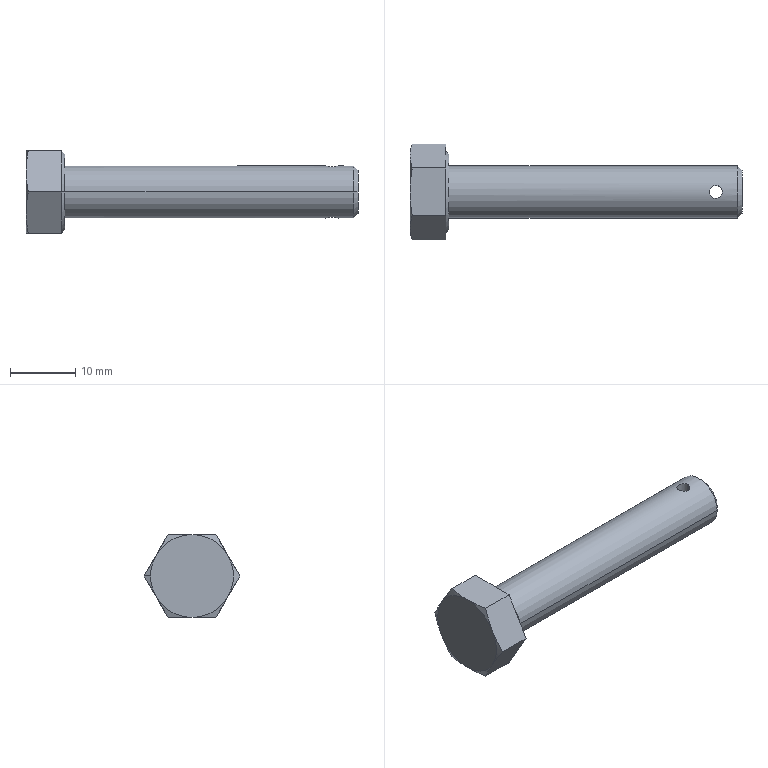Part | SolidWorks | features BaseBody 1 | 1 solid | 30 faces | box 50.95 x 14.699 x 12.73 mm | volume 3053 mm3 | plane 15 | cone 11 | cylinder 4 | commonest cylinder face diameters 2 x2 8 x2
STEP:
#1=CARTESIAN_POINT('',(45.95,0.,-4.));
#2=VERTEX_POINT('',#1);
#3=CARTESIAN_POINT('',(47.95,0.,-4.));
#4=VERTEX_POINT('',#3);
#5=CARTESIAN_POINT('',(45.95,0.,-4.));
#6=CARTESIAN_POINT('',(45.95,-0.1327,-4.));
#7=CARTESIAN_POINT('',(45.976,-0.2612,-3.993));
#8=CARTESIAN_POINT('',(46.077,-0.5055,-3.97));
#9=CARTESIAN_POINT('',(46.149,-0.6129,-3.954));
#10=CARTESIAN_POINT('',(46.336,-0.8007,-3.92));
#11=CARTESIAN_POINT('',(46.443,-0.8722,-3.904));
#12=CARTESIAN_POINT('',(46.689,-0.9745,-3.88));
#13=CARTESIAN_POINT('',(46.817,-0.9999,-3.873));
#14=CARTESIAN_POINT('',(47.082,-1.,-3.873));
#15=CARTESIAN_POINT('',(47.212,-0.9741,-3.88));
#16=CARTESIAN_POINT('',(47.455,-0.8731,-3.904));
#17=CARTESIAN_POINT('',(47.563,-0.8008,-3.92));
#18=CARTESIAN_POINT('',(47.75,-0.6142,-3.954));
#19=CARTESIAN_POINT('',(47.822,-0.5075,-3.97));
#20=CARTESIAN_POINT('',(47.924,-0.2615,-3.993));
#21=CARTESIAN_POINT('',(47.95,-0.1331,-4.));
#22=CARTESIAN_POINT('',(47.95,0.,-4.));
#23=B_SPLINE_CURVE_WITH_KNOTS('',3,(#5,#6,#7,#8,#9,#10,#11,#12,#13,#14,#15,#16,#17,#18,#19,#20,#21,#22),.UNSPECIFIED.,.F.,.F.,(4,2,2,2,2,2,2,2,4),(0.,0.125,0.25,0.375,0.5,0.625,0.75,0.875,1.),.UNSPECIFIED.);
#24=EDGE_CURVE('',#2,#4,#23,.T.);
#25=ORIENTED_EDGE('',*,*,#24,.F.);
#26=CARTESIAN_POINT('',(45.95,0.,4.));
#27=VERTEX_POINT('',#26);
#28=CARTESIAN_POINT('',(45.95,0.,-6.365));
#29=DIRECTION('',(0.,0.,1.));
#30=VECTOR('',#29,1000.);
#31=LINE('',#28,#30);
#32=EDGE_CURVE('',#2,#27,#31,.T.);
#33=ORIENTED_EDGE('',*,*,#32,.T.);
#34=CARTESIAN_POINT('',(47.95,0.,4.));
#35=VERTEX_POINT('',#34);
#36=CARTESIAN_POINT('',(47.95,0.,4.));
#37=CARTESIAN_POINT('',(47.95,-0.1329,4.));
#38=CARTESIAN_POINT('',(47.924,-0.2617,3.993));
#39=CARTESIAN_POINT('',(47.823,-0.5061,3.97));
#40=CARTESIAN_POINT('',(47.751,-0.6136,3.954));
#41=CARTESIAN_POINT('',(47.563,-0.8011,3.92));
#42=CARTESIAN_POINT('',(47.456,-0.8725,3.904));
#43=CARTESIAN_POINT('',(47.211,-0.9745,3.88));
#44=CARTESIAN_POINT('',(47.083,-0.9999,3.873));
#45=CARTESIAN_POINT('',(46.818,-1.,3.873));
#46=CARTESIAN_POINT('',(46.689,-0.9742,3.88));
#47=CARTESIAN_POINT('',(46.445,-0.873,3.904));
#48=CARTESIAN_POINT('',(46.336,-0.8005,3.92));
#49=CARTESIAN_POINT('',(46.149,-0.6134,3.954));
#50=CARTESIAN_POINT('',(46.077,-0.506,3.97));
#51=CARTESIAN_POINT('',(45.975,-0.2607,3.993));
#52=CARTESIAN_POINT('',(45.95,-0.1327,4.));
#53=CARTESIAN_POINT('',(45.95,0.,4.));
#54=B_SPLINE_CURVE_WITH_KNOTS('',3,(#36,#37,#38,#39,#40,#41,#42,#43,#44,#45,#46,#47,#48,#49,#50,#51,#52,#53),.UNSPECIFIED.,.F.,.F.,(4,2,2,2,2,2,2,2,4),(0.,0.125,0.25,0.375,0.5,0.625,0.75,0.875,1.),.UNSPECIFIED.);
#55=EDGE_CURVE('',#35,#27,#54,.T.);
#56=ORIENTED_EDGE('',*,*,#55,.F.);
#57=CARTESIAN_POINT('',(47.95,0.,-6.365));
#58=DIRECTION('',(0.,0.,1.));
#59=VECTOR('',#58,1000.);
#60=LINE('',#57,#59);
#61=EDGE_CURVE('',#4,#35,#60,.T.);
#62=ORIENTED_EDGE('',*,*,#61,.F.);
#63=EDGE_LOOP('',(#25,#33,#56,#62));
#64=FACE_OUTER_BOUND('',#63,.T.);
#65=CARTESIAN_POINT('',(46.95,0.,-6.365));
#66=DIRECTION('',(0.,0.,1.));
#67=DIRECTION('',(1.,0.,0.));
#68=AXIS2_PLACEMENT_3D('',#65,#66,#67);
#69=CYLINDRICAL_SURFACE('',#68,1.);
#70=ADVANCED_FACE('',(#64),#69,.F.);
#71=CARTESIAN_POINT('',(50.95,3.324,0.));
#72=VERTEX_POINT('',#71);
#73=CARTESIAN_POINT('',(50.95,-3.324,0.));
#74=VERTEX_POINT('',#73);
#75=CARTESIAN_POINT('',(50.95,0.,0.));
#76=DIRECTION('',(1.,0.,0.));
#77=DIRECTION('',(0.,1.,0.));
#78=AXIS2_PLACEMENT_3D('',#75,#76,#77);
#79=CIRCLE('',#78,3.324);
#80=EDGE_CURVE('',#72,#74,#79,.T.);
#81=ORIENTED_EDGE('',*,*,#80,.F.);
#82=CARTESIAN_POINT('',(50.273,4.,0.));
#83=VERTEX_POINT('',#82);
#84=CARTESIAN_POINT('',(50.95,3.324,0.));
#85=DIRECTION('',(-0.7071,0.7071,0.));
#86=VECTOR('',#85,1000.);
#87=LINE('',#84,#86);
#88=EDGE_CURVE('',#72,#83,#87,.T.);
#89=ORIENTED_EDGE('',*,*,#88,.T.);
#90=CARTESIAN_POINT('',(50.273,-4.,0.));
#91=VERTEX_POINT('',#90);
#92=CARTESIAN_POINT('',(50.273,0.,0.));
#93=DIRECTION('',(-1.,0.,0.));
#94=DIRECTION('',(0.,1.,0.));
#95=AXIS2_PLACEMENT_3D('',#92,#93,#94);
#96=CIRCLE('',#95,4.);
#97=EDGE_CURVE('',#91,#83,#96,.T.);
#98=ORIENTED_EDGE('',*,*,#97,.F.);
#99=CARTESIAN_POINT('',(50.95,-3.324,0.));
#100=DIRECTION('',(-0.7071,-0.7071,0.));
#101=VECTOR('',#100,1000.);
#102=LINE('',#99,#101);
#103=EDGE_CURVE('',#74,#91,#102,.T.);
#104=ORIENTED_EDGE('',*,*,#103,.F.);
#105=EDGE_LOOP('',(#81,#89,#98,#104));
#106=FACE_OUTER_BOUND('',#105,.T.);
#107=CARTESIAN_POINT('',(50.95,0.,0.));
#108=DIRECTION('',(-1.,0.,0.));
#109=DIRECTION('',(0.,-1.,0.));
#110=AXIS2_PLACEMENT_3D('',#107,#108,#109);
#111=CONICAL_SURFACE('',#110,3.324,0.7854);
#112=ADVANCED_FACE('',(#106),#111,.T.);
#113=ORIENTED_EDGE('',*,*,#97,.T.);
#114=CARTESIAN_POINT('',(5.95,4.,0.));
#115=VERTEX_POINT('',#114);
#116=CARTESIAN_POINT('',(50.95,4.,0.));
#117=DIRECTION('',(-1.,0.,0.));
#118=VECTOR('',#117,1000.);
#119=LINE('',#116,#118);
#120=EDGE_CURVE('',#83,#115,#119,.T.);
#121=ORIENTED_EDGE('',*,*,#120,.T.);
#122=CARTESIAN_POINT('',(5.95,-4.,0.));
#123=VERTEX_POINT('',#122);
#124=CARTESIAN_POINT('',(5.95,0.,0.));
#125=DIRECTION('',(1.,0.,0.));
#126=DIRECTION('',(0.,-1.,0.));
#127=AXIS2_PLACEMENT_3D('',#124,#125,#126);
#128=CIRCLE('',#127,4.);
#129=EDGE_CURVE('',#115,#123,#128,.T.);
#130=ORIENTED_EDGE('',*,*,#129,.T.);
#131=CARTESIAN_POINT('',(50.95,-4.,0.));
#132=DIRECTION('',(-1.,0.,0.));
#133=VECTOR('',#132,1000.);
#134=LINE('',#131,#133);
#135=EDGE_CURVE('',#91,#123,#134,.T.);
#136=ORIENTED_EDGE('',*,*,#135,.F.);
#137=EDGE_LOOP('',(#113,#121,#130,#136));
#138=FACE_OUTER_BOUND('',#137,.T.);
#139=ORIENTED_EDGE('',*,*,#55,.T.);
#140=CARTESIAN_POINT('',(45.95,0.,4.));
#141=CARTESIAN_POINT('',(45.95,0.1327,4.));
#142=CARTESIAN_POINT('',(45.976,0.2612,3.993));
#143=CARTESIAN_POINT('',(46.077,0.5055,3.97));
#144=CARTESIAN_POINT('',(46.149,0.6129,3.954));
#145=CARTESIAN_POINT('',(46.336,0.8007,3.92));
#146=CARTESIAN_POINT('',(46.443,0.8722,3.904));
#147=CARTESIAN_POINT('',(46.689,0.9745,3.88));
#148=CARTESIAN_POINT('',(46.817,0.9999,3.873));
#149=CARTESIAN_POINT('',(47.082,1.,3.873));
#150=CARTESIAN_POINT('',(47.212,0.9741,3.88));
#151=CARTESIAN_POINT('',(47.455,0.8731,3.904));
#152=CARTESIAN_POINT('',(47.563,0.8008,3.92));
#153=CARTESIAN_POINT('',(47.75,0.6142,3.954));
#154=CARTESIAN_POINT('',(47.822,0.5075,3.97));
#155=CARTESIAN_POINT('',(47.924,0.2615,3.993));
#156=CARTESIAN_POINT('',(47.95,0.1331,4.));
#157=CARTESIAN_POINT('',(47.95,0.,4.));
#158=B_SPLINE_CURVE_WITH_KNOTS('',3,(#140,#141,#142,#143,#144,#145,#146,#147,#148,#149,#150,#151,#152,#153,#154,#155,#156,#157),.UNSPECIFIED.,.F.,.F.,(4,2,2,2,2,2,2,2,4),(0.,0.125,0.25,0.375,0.5,0.625,0.75,0.875,1.),.UNSPECIFIED.);
#159=EDGE_CURVE('',#27,#35,#158,.T.);
#160=ORIENTED_EDGE('',*,*,#159,.T.);
#161=EDGE_LOOP('',(#139,#160));
#162=FACE_BOUND('',#161,.T.);
#163=CARTESIAN_POINT('',(50.95,0.,0.));
#164=DIRECTION('',(-1.,0.,0.));
#165=DIRECTION('',(0.,-1.,0.));
#166=AXIS2_PLACEMENT_3D('',#163,#164,#165);
#167=CYLINDRICAL_SURFACE('',#166,4.);
#168=ADVANCED_FACE('',(#138,#162),#167,.T.);
#169=CARTESIAN_POINT('',(5.95,-5.815,0.));
#170=VERTEX_POINT('',#169);
#171=CARTESIAN_POINT('',(5.95,5.815,0.));
#172=VERTEX_POINT('',#171);
#173=CARTESIAN_POINT('',(5.95,0.,0.));
#174=DIRECTION('',(-1.,0.,0.));
#175=DIRECTION('',(0.,-1.,0.));
#176=AXIS2_PLACEMENT_3D('',#173,#174,#175);
#177=CIRCLE('',#176,5.815);
#178=EDGE_CURVE('',#170,#172,#177,.T.);
#179=ORIENTED_EDGE('',*,*,#178,.T.);
#180=CARTESIAN_POINT('',(5.45,6.365,0.));
#181=VERTEX_POINT('',#180);
#182=CARTESIAN_POINT('',(5.95,5.815,0.));
#183=DIRECTION('',(-0.6727,0.7399,0.));
#184=VECTOR('',#183,1000.);
#185=LINE('',#182,#184);
#186=EDGE_CURVE('',#172,#181,#185,.T.);
#187=ORIENTED_EDGE('',*,*,#186,.T.);
#188=CARTESIAN_POINT('',(5.45,5.512,3.183));
#189=VERTEX_POINT('',#188);
#190=CARTESIAN_POINT('',(5.45,0.,0.));
#191=DIRECTION('',(-1.,0.,0.));
#192=DIRECTION('',(0.,-1.,0.));
#193=AXIS2_PLACEMENT_3D('',#190,#191,#192);
#194=CIRCLE('',#193,6.365);
#195=EDGE_CURVE('',#189,#181,#194,.T.);
#196=ORIENTED_EDGE('',*,*,#195,.F.);
#197=CARTESIAN_POINT('',(5.45,0.,6.365));
#198=VERTEX_POINT('',#197);
#199=CARTESIAN_POINT('',(5.45,0.,0.));
#200=DIRECTION('',(-1.,0.,0.));
#201=DIRECTION('',(0.,-1.,0.));
#202=AXIS2_PLACEMENT_3D('',#199,#200,#201);
#203=CIRCLE('',#202,6.365);
#204=EDGE_CURVE('',#198,#189,#203,.T.);
#205=ORIENTED_EDGE('',*,*,#204,.F.);
#206=CARTESIAN_POINT('',(5.45,-5.512,3.183));
#207=VERTEX_POINT('',#206);
#208=CARTESIAN_POINT('',(5.45,0.,0.));
#209=DIRECTION('',(-1.,0.,0.));
#210=DIRECTION('',(0.,-1.,0.));
#211=AXIS2_PLACEMENT_3D('',#208,#209,#210);
#212=CIRCLE('',#211,6.365);
#213=EDGE_CURVE('',#207,#198,#212,.T.);
#214=ORIENTED_EDGE('',*,*,#213,.F.);
#215=CARTESIAN_POINT('',(5.45,-6.365,0.));
#216=VERTEX_POINT('',#215);
#217=CARTESIAN_POINT('',(5.45,0.,0.));
#218=DIRECTION('',(-1.,0.,0.));
#219=DIRECTION('',(0.,-1.,0.));
#220=AXIS2_PLACEMENT_3D('',#217,#218,#219);
#221=CIRCLE('',#220,6.365);
#222=EDGE_CURVE('',#216,#207,#221,.T.);
#223=ORIENTED_EDGE('',*,*,#222,.F.);
#224=CARTESIAN_POINT('',(5.95,-5.815,0.));
#225=DIRECTION('',(-0.6727,-0.7399,0.));
#226=VECTOR('',#225,1000.);
#227=LINE('',#224,#226);
#228=EDGE_CURVE('',#170,#216,#227,.T.);
#229=ORIENTED_EDGE('',*,*,#228,.F.);
#230=EDGE_LOOP('',(#179,#187,#196,#205,#214,#223,#229));
#231=FACE_OUTER_BOUND('',#230,.T.);
#232=CARTESIAN_POINT('',(5.95,0.,0.));
#233=DIRECTION('',(-1.,0.,0.));
#234=DIRECTION('',(0.,-1.,0.));
#235=AXIS2_PLACEMENT_3D('',#232,#233,#234);
#236=CONICAL_SURFACE('',#235,5.815,0.833);
#237=ADVANCED_FACE('',(#231),#236,.T.);
#238=CARTESIAN_POINT('',(0.,6.365,0.));
#239=VERTEX_POINT('',#238);
#240=CARTESIAN_POINT('',(0.,5.512,-3.183));
#241=VERTEX_POINT('',#240);
#242=CARTESIAN_POINT('',(0.,0.,0.));
#243=DIRECTION('',(-1.,0.,0.));
#244=DIRECTION('',(0.,0.,1.));
#245=AXIS2_PLACEMENT_3D('',#242,#243,#244);
#246=CIRCLE('',#245,6.365);
#247=EDGE_CURVE('',#239,#241,#246,.T.);
#248=ORIENTED_EDGE('',*,*,#247,.F.);
#249=CARTESIAN_POINT('',(0.3584,7.35,0.));
#250=VERTEX_POINT('',#249);
#251=CARTESIAN_POINT('',(0.,6.365,0.));
#252=DIRECTION('',(0.342,0.9397,0.));
#253=VECTOR('',#252,1000.);
#254=LINE('',#251,#253);
#255=EDGE_CURVE('',#239,#250,#254,.T.);
#256=ORIENTED_EDGE('',*,*,#255,.T.);
#257=CARTESIAN_POINT('',(0.3584,7.35,0.));
#258=CARTESIAN_POINT('',(0.3008,7.191,-0.2742));
#259=CARTESIAN_POINT('',(0.25,7.037,-0.5421));
#260=CARTESIAN_POINT('',(0.184,6.808,-0.9385));
#261=CARTESIAN_POINT('',(0.1638,6.732,-1.07));
#262=CARTESIAN_POINT('',(0.1359,6.619,-1.266));
#263=CARTESIAN_POINT('',(0.127,6.581,-1.331));
#264=CARTESIAN_POINT('',(0.1102,6.506,-1.461));
#265=CARTESIAN_POINT('',(0.1024,6.47,-1.524));
#266=CARTESIAN_POINT('',(0.07901,6.354,-1.725));
#267=CARTESIAN_POINT('',(0.06534,6.277,-1.858));
#268=CARTESIAN_POINT('',(0.04182,6.124,-2.123));
#269=CARTESIAN_POINT('',(0.03203,6.049,-2.254));
#270=CARTESIAN_POINT('',(0.008007,5.818,-2.654));
#271=CARTESIAN_POINT('',(0.,5.666,-2.917));
#272=CARTESIAN_POINT('',(0.,5.512,-3.183));
#273=B_SPLINE_CURVE_WITH_KNOTS('',3,(#257,#258,#259,#260,#261,#262,#263,#264,#265,#266,#267,#268,#269,#270,#271,#272),.UNSPECIFIED.,.F.,.F.,(4,2,2,2,2,2,2,4),(0.,0.25,0.375,0.4375,0.5,0.625,0.75,1.),.UNSPECIFIED.);
#274=EDGE_CURVE('',#250,#241,#273,.T.);
#275=ORIENTED_EDGE('',*,*,#274,.T.);
#276=EDGE_LOOP('',(#248,#256,#275));
#277=FACE_OUTER_BOUND('',#276,.T.);
#278=CARTESIAN_POINT('',(0.,0.,0.));
#279=DIRECTION('',(1.,0.,0.));
#280=DIRECTION('',(0.,1.,0.));
#281=AXIS2_PLACEMENT_3D('',#278,#279,#280);
#282=CONICAL_SURFACE('',#281,6.365,1.222);
#283=ADVANCED_FACE('',(#277),#282,.T.);
#284=ORIENTED_EDGE('',*,*,#178,.F.);
#285=CARTESIAN_POINT('',(5.95,0.,0.));
#286=DIRECTION('',(-1.,0.,0.));
#287=DIRECTION('',(0.,-1.,0.));
#288=AXIS2_PLACEMENT_3D('',#285,#286,#287);
#289=CIRCLE('',#288,5.815);
#290=EDGE_CURVE('',#172,#170,#289,.T.);
#291=ORIENTED_EDGE('',*,*,#290,.F.);
#292=EDGE_LOOP('',(#284,#291));
#293=FACE_OUTER_BOUND('',#292,.T.);
#294=CARTESIAN_POINT('',(5.95,0.,0.));
#295=DIRECTION('',(1.,0.,0.));
#296=DIRECTION('',(0.,-1.,0.));
#297=AXIS2_PLACEMENT_3D('',#294,#295,#296);
#298=CIRCLE('',#297,4.);
#299=EDGE_CURVE('',#123,#115,#298,.T.);
#300=ORIENTED_EDGE('',*,*,#299,.F.);
#301=ORIENTED_EDGE('',*,*,#129,.F.);
#302=EDGE_LOOP('',(#300,#301));
#303=FACE_BOUND('',#302,.T.);
#304=CARTESIAN_POINT('',(5.95,0.,0.));
#305=DIRECTION('',(-1.,0.,0.));
#306=DIRECTION('',(0.,1.,0.));
#307=AXIS2_PLACEMENT_3D('',#304,#305,#306);
#308=PLANE('',#307);
#309=ADVANCED_FACE('',(#293,#303),#308,.F.);
#310=CARTESIAN_POINT('',(5.45,-3.675,6.365));
#311=VERTEX_POINT('',#310);
#312=CARTESIAN_POINT('',(5.45,-3.675,6.365));
#313=DIRECTION('',(0.,-0.5,-0.866));
#314=VECTOR('',#313,1000.);
#315=LINE('',#312,#314);
#316=EDGE_CURVE('',#311,#207,#315,.T.);
#317=ORIENTED_EDGE('',*,*,#316,.T.);
#318=ORIENTED_EDGE('',*,*,#213,.T.);
#319=CARTESIAN_POINT('',(5.45,3.675,6.365));
#320=DIRECTION('',(0.,-1.,0.));
#321=VECTOR('',#320,1000.);
#322=LINE('',#319,#321);
#323=EDGE_CURVE('',#198,#311,#322,.T.);
#324=ORIENTED_EDGE('',*,*,#323,.T.);
#325=EDGE_LOOP('',(#317,#318,#324));
#326=FACE_OUTER_BOUND('',#325,.T.);
#327=CARTESIAN_POINT('',(5.45,0.,12.73));
#328=DIRECTION('',(-1.,0.,0.));
#329=DIRECTION('',(0.,0.,1.));
#330=AXIS2_PLACEMENT_3D('',#327,#328,#329);
#331=PLANE('',#330);
#332=ADVANCED_FACE('',(#326),#331,.F.);
#333=CARTESIAN_POINT('',(5.45,3.675,6.365));
#334=VERTEX_POINT('',#333);
#335=CARTESIAN_POINT('',(5.45,3.675,6.365));
#336=DIRECTION('',(0.,-1.,0.));
#337=VECTOR('',#336,1000.);
#338=LINE('',#335,#337);
#339=EDGE_CURVE('',#334,#198,#338,.T.);
#340=ORIENTED_EDGE('',*,*,#339,.T.);
#341=ORIENTED_EDGE('',*,*,#204,.T.);
#342=CARTESIAN_POINT('',(5.45,7.35,0.));
#343=DIRECTION('',(0.,-0.5,0.866));
#344=VECTOR('',#343,1000.);
#345=LINE('',#342,#344);
#346=EDGE_CURVE('',#189,#334,#345,.T.);
#347=ORIENTED_EDGE('',*,*,#346,.T.);
#348=EDGE_LOOP('',(#340,#341,#347));
#349=FACE_OUTER_BOUND('',#348,.T.);
#350=CARTESIAN_POINT('',(5.45,0.,12.73));
#351=DIRECTION('',(-1.,0.,0.));
#352=DIRECTION('',(0.,0.,1.));
#353=AXIS2_PLACEMENT_3D('',#350,#351,#352);
#354=PLANE('',#353);
#355=ADVANCED_FACE('',(#349),#354,.F.);
#356=CARTESIAN_POINT('',(5.45,7.35,0.));
#357=VERTEX_POINT('',#356);
#358=CARTESIAN_POINT('',(5.45,7.35,0.));
#359=DIRECTION('',(0.,-0.5,0.866));
#360=VECTOR('',#359,1000.);
#361=LINE('',#358,#360);
#362=EDGE_CURVE('',#357,#189,#361,.T.);
#363=ORIENTED_EDGE('',*,*,#362,.T.);
#364=ORIENTED_EDGE('',*,*,#195,.T.);
#365=CARTESIAN_POINT('',(5.45,5.512,-3.183));
#366=VERTEX_POINT('',#365);
#367=CARTESIAN_POINT('',(5.45,0.,0.));
#368=DIRECTION('',(-1.,0.,0.));
#369=DIRECTION('',(0.,-1.,0.));
#370=AXIS2_PLACEMENT_3D('',#367,#368,#369);
#371=CIRCLE('',#370,6.365);
#372=EDGE_CURVE('',#181,#366,#371,.T.);
#373=ORIENTED_EDGE('',*,*,#372,.T.);
#374=CARTESIAN_POINT('',(5.45,3.675,-6.365));
#375=DIRECTION('',(0.,0.5,0.866));
#376=VECTOR('',#375,1000.);
#377=LINE('',#374,#376);
#378=EDGE_CURVE('',#366,#357,#377,.T.);
#379=ORIENTED_EDGE('',*,*,#378,.T.);
#380=EDGE_LOOP('',(#363,#364,#373,#379));
#381=FACE_OUTER_BOUND('',#380,.T.);
#382=CARTESIAN_POINT('',(5.45,0.,12.73));
#383=DIRECTION('',(-1.,0.,0.));
#384=DIRECTION('',(0.,0.,1.));
#385=AXIS2_PLACEMENT_3D('',#382,#383,#384);
#386=PLANE('',#385);
#387=ADVANCED_FACE('',(#381),#386,.F.);
#388=CARTESIAN_POINT('',(5.45,3.675,-6.365));
#389=VERTEX_POINT('',#388);
#390=CARTESIAN_POINT('',(5.45,3.675,-6.365));
#391=DIRECTION('',(0.,0.5,0.866));
#392=VECTOR('',#391,1000.);
#393=LINE('',#390,#392);
#394=EDGE_CURVE('',#389,#366,#393,.T.);
#395=ORIENTED_EDGE('',*,*,#394,.T.);
#396=CARTESIAN_POINT('',(5.45,0.,-6.365));
#397=VERTEX_POINT('',#396);
#398=CARTESIAN_POINT('',(5.45,0.,0.));
#399=DIRECTION('',(-1.,0.,0.));
#400=DIRECTION('',(0.,-1.,0.));
#401=AXIS2_PLACEMENT_3D('',#398,#399,#400);
#402=CIRCLE('',#401,6.365);
#403=EDGE_CURVE('',#366,#397,#402,.T.);
#404=ORIENTED_EDGE('',*,*,#403,.T.);
#405=CARTESIAN_POINT('',(5.45,-3.675,-6.365));
#406=DIRECTION('',(0.,1.,0.));
#407=VECTOR('',#406,1000.);
#408=LINE('',#405,#407);
#409=EDGE_CURVE('',#397,#389,#408,.T.);
#410=ORIENTED_EDGE('',*,*,#409,.T.);
#411=EDGE_LOOP('',(#395,#404,#410));
#412=FACE_OUTER_BOUND('',#411,.T.);
#413=CARTESIAN_POINT('',(5.45,0.,12.73));
#414=DIRECTION('',(-1.,0.,0.));
#415=DIRECTION('',(0.,0.,1.));
#416=AXIS2_PLACEMENT_3D('',#413,#414,#415);
#417=PLANE('',#416);
#418=ADVANCED_FACE('',(#412),#417,.F.);
#419=CARTESIAN_POINT('',(5.45,-3.675,-6.365));
#420=VERTEX_POINT('',#419);
#421=CARTESIAN_POINT('',(5.45,-3.675,-6.365));
#422=DIRECTION('',(0.,1.,0.));
#423=VECTOR('',#422,1000.);
#424=LINE('',#421,#423);
#425=EDGE_CURVE('',#420,#397,#424,.T.);
#426=ORIENTED_EDGE('',*,*,#425,.T.);
#427=CARTESIAN_POINT('',(5.45,-5.512,-3.183));
#428=VERTEX_POINT('',#427);
#429=CARTESIAN_POINT('',(5.45,0.,0.));
#430=DIRECTION('',(-1.,0.,0.));
#431=DIRECTION('',(0.,-1.,0.));
#432=AXIS2_PLACEMENT_3D('',#429,#430,#431);
#433=CIRCLE('',#432,6.365);
#434=EDGE_CURVE('',#397,#428,#433,.T.);
#435=ORIENTED_EDGE('',*,*,#434,.T.);
#436=CARTESIAN_POINT('',(5.45,-7.35,0.));
#437=DIRECTION('',(0.,0.5,-0.866));
#438=VECTOR('',#437,1000.);
#439=LINE('',#436,#438);
#440=EDGE_CURVE('',#428,#420,#439,.T.);
#441=ORIENTED_EDGE('',*,*,#440,.T.);
#442=EDGE_LOOP('',(#426,#435,#441));
#443=FACE_OUTER_BOUND('',#442,.T.);
#444=CARTESIAN_POINT('',(5.45,0.,12.73));
#445=DIRECTION('',(-1.,0.,0.));
#446=DIRECTION('',(0.,0.,1.));
#447=AXIS2_PLACEMENT_3D('',#444,#445,#446);
#448=PLANE('',#447);
#449=ADVANCED_FACE('',(#443),#448,.F.);
#450=CARTESIAN_POINT('',(0.3584,-7.35,0.));
#451=VERTEX_POINT('',#450);
#452=CARTESIAN_POINT('',(0.,-5.512,3.183));
#453=VERTEX_POINT('',#452);
#454=CARTESIAN_POINT('',(0.3584,-7.35,0.));
#455=CARTESIAN_POINT('',(0.3008,-7.191,0.2742));
#456=CARTESIAN_POINT('',(0.25,-7.037,0.5421));
#457=CARTESIAN_POINT('',(0.184,-6.808,0.9385));
#458=CARTESIAN_POINT('',(0.1638,-6.732,1.07));
#459=CARTESIAN_POINT('',(0.1359,-6.619,1.266));
#460=CARTESIAN_POINT('',(0.127,-6.581,1.331));
#461=CARTESIAN_POINT('',(0.1102,-6.506,1.461));
#462=CARTESIAN_POINT('',(0.1024,-6.47,1.524));
#463=CARTESIAN_POINT('',(0.07901,-6.354,1.725));
#464=CARTESIAN_POINT('',(0.06534,-6.277,1.858));
#465=CARTESIAN_POINT('',(0.04182,-6.124,2.123));
#466=CARTESIAN_POINT('',(0.03203,-6.049,2.254));
#467=CARTESIAN_POINT('',(0.008007,-5.818,2.654));
#468=CARTESIAN_POINT('',(0.,-5.666,2.917));
#469=CARTESIAN_POINT('',(0.,-5.512,3.183));
#470=B_SPLINE_CURVE_WITH_KNOTS('',3,(#454,#455,#456,#457,#458,#459,#460,#461,#462,#463,#464,#465,#466,#467,#468,#469),.UNSPECIFIED.,.F.,.F.,(4,2,2,2,2,2,2,4),(0.,0.25,0.375,0.4375,0.5,0.625,0.75,1.),.UNSPECIFIED.);
#471=EDGE_CURVE('',#451,#453,#470,.T.);
#472=ORIENTED_EDGE('',*,*,#471,.F.);
#473=CARTESIAN_POINT('',(5.45,-7.35,0.));
#474=VERTEX_POINT('',#473);
#475=CARTESIAN_POINT('',(5.45,-7.35,0.));
#476=DIRECTION('',(-1.,0.,0.));
#477=VECTOR('',#476,1000.);
#478=LINE('',#475,#477);
#479=EDGE_CURVE('',#474,#451,#478,.T.);
#480=ORIENTED_EDGE('',*,*,#479,.F.);
#481=CARTESIAN_POINT('',(5.45,-3.675,6.365));
#482=DIRECTION('',(0.,-0.5,-0.866));
#483=VECTOR('',#482,1000.);
#484=LINE('',#481,#483);
#485=EDGE_CURVE('',#207,#474,#484,.T.);
#486=ORIENTED_EDGE('',*,*,#485,.F.);
#487=ORIENTED_EDGE('',*,*,#316,.F.);
#488=CARTESIAN_POINT('',(0.3584,-3.675,6.365));
#489=VERTEX_POINT('',#488);
#490=CARTESIAN_POINT('',(5.45,-3.675,6.365));
#491=DIRECTION('',(-1.,0.,0.));
#492=VECTOR('',#491,1000.);
#493=LINE('',#490,#492);
#494=EDGE_CURVE('',#311,#489,#493,.T.);
#495=ORIENTED_EDGE('',*,*,#494,.T.);
#496=CARTESIAN_POINT('',(0.,-5.512,3.183));
#497=CARTESIAN_POINT('',(0.,-5.436,3.315));
#498=CARTESIAN_POINT('',(0.002002,-5.359,3.447));
#499=CARTESIAN_POINT('',(0.01001,-5.206,3.712));
#500=CARTESIAN_POINT('',(0.01608,-5.129,3.846));
#501=CARTESIAN_POINT('',(0.03196,-4.977,4.11));
#502=CARTESIAN_POINT('',(0.04181,-4.9,4.242));
#503=CARTESIAN_POINT('',(0.05946,-4.786,4.441));
#504=CARTESIAN_POINT('',(0.06582,-4.747,4.507));
#505=CARTESIAN_POINT('',(0.07949,-4.671,4.64));
#506=CARTESIAN_POINT('',(0.08702,-4.631,4.709));
#507=CARTESIAN_POINT('',(0.1552,-4.293,5.294));
#508=CARTESIAN_POINT('',(0.2431,-3.991,5.817));
#509=CARTESIAN_POINT('',(0.3584,-3.675,6.365));
#510=B_SPLINE_CURVE_WITH_KNOTS('',3,(#496,#497,#498,#499,#500,#501,#502,#503,#504,#505,#506,#507,#508,#509),.UNSPECIFIED.,.F.,.F.,(4,2,2,2,2,2,4),(0.,0.125,0.25,0.375,0.4375,0.5,1.),.UNSPECIFIED.);
#511=EDGE_CURVE('',#453,#489,#510,.T.);
#512=ORIENTED_EDGE('',*,*,#511,.F.);
#513=EDGE_LOOP('',(#472,#480,#486,#487,#495,#512));
#514=FACE_OUTER_BOUND('',#513,.T.);
#515=CARTESIAN_POINT('',(5.45,-3.675,6.365));
#516=DIRECTION('',(0.,0.866,-0.5));
#517=DIRECTION('',(-1.,0.,0.));
#518=AXIS2_PLACEMENT_3D('',#515,#516,#517);
#519=PLANE('',#518);
#520=ADVANCED_FACE('',(#514),#519,.F.);
#521=CARTESIAN_POINT('',(0.3584,-3.675,-6.365));
#522=VERTEX_POINT('',#521);
#523=CARTESIAN_POINT('',(0.,-5.512,-3.183));
#524=VERTEX_POINT('',#523);
#525=CARTESIAN_POINT('',(0.3584,-3.675,-6.365));
#526=CARTESIAN_POINT('',(0.3008,-3.833,-6.091));
#527=CARTESIAN_POINT('',(0.25,-3.988,-5.823));
#528=CARTESIAN_POINT('',(0.184,-4.217,-5.426));
#529=CARTESIAN_POINT('',(0.1638,-4.292,-5.295));
#530=CARTESIAN_POINT('',(0.1359,-4.406,-5.099));
#531=CARTESIAN_POINT('',(0.127,-4.443,-5.034));
#532=CARTESIAN_POINT('',(0.1102,-4.518,-4.904));
#533=CARTESIAN_POINT('',(0.1024,-4.555,-4.841));
#534=CARTESIAN_POINT('',(0.07901,-4.671,-4.64));
#535=CARTESIAN_POINT('',(0.06534,-4.747,-4.507));
#536=CARTESIAN_POINT('',(0.04182,-4.9,-4.242));
#537=CARTESIAN_POINT('',(0.03203,-4.976,-4.111));
#538=CARTESIAN_POINT('',(0.008007,-5.207,-3.711));
#539=CARTESIAN_POINT('',(0.,-5.359,-3.448));
#540=CARTESIAN_POINT('',(0.,-5.512,-3.183));
#541=B_SPLINE_CURVE_WITH_KNOTS('',3,(#525,#526,#527,#528,#529,#530,#531,#532,#533,#534,#535,#536,#537,#538,#539,#540),.UNSPECIFIED.,.F.,.F.,(4,2,2,2,2,2,2,4),(0.,0.25,0.375,0.4375,0.5,0.625,0.75,1.),.UNSPECIFIED.);
#542=EDGE_CURVE('',#522,#524,#541,.T.);
#543=ORIENTED_EDGE('',*,*,#542,.F.);
#544=CARTESIAN_POINT('',(5.45,-3.675,-6.365));
#545=DIRECTION('',(-1.,0.,0.));
#546=VECTOR('',#545,1000.);
#547=LINE('',#544,#546);
#548=EDGE_CURVE('',#420,#522,#547,.T.);
#549=ORIENTED_EDGE('',*,*,#548,.F.);
#550=ORIENTED_EDGE('',*,*,#440,.F.);
#551=CARTESIAN_POINT('',(5.45,-7.35,0.));
#552=DIRECTION('',(0.,0.5,-0.866));
#553=VECTOR('',#552,1000.);
#554=LINE('',#551,#553);
#555=EDGE_CURVE('',#474,#428,#554,.T.);
#556=ORIENTED_EDGE('',*,*,#555,.F.);
#557=ORIENTED_EDGE('',*,*,#479,.T.);
#558=CARTESIAN_POINT('',(0.,-5.512,-3.183));
#559=CARTESIAN_POINT('',(0.,-5.589,-3.05));
#560=CARTESIAN_POINT('',(0.002002,-5.665,-2.918));
#561=CARTESIAN_POINT('',(0.01001,-5.818,-2.653));
#562=CARTESIAN_POINT('',(0.01608,-5.895,-2.519));
#563=CARTESIAN_POINT('',(0.03196,-6.048,-2.255));
#564=CARTESIAN_POINT('',(0.04181,-6.124,-2.123));
#565=CARTESIAN_POINT('',(0.05946,-6.239,-1.924));
#566=CARTESIAN_POINT('',(0.06582,-6.277,-1.858));
#567=CARTESIAN_POINT('',(0.07949,-6.354,-1.725));
#568=CARTESIAN_POINT('',(0.08702,-6.393,-1.656));
#569=CARTESIAN_POINT('',(0.1552,-6.731,-1.071));
#570=CARTESIAN_POINT('',(0.2431,-7.033,-0.5484));
#571=CARTESIAN_POINT('',(0.3584,-7.35,0.));
#572=B_SPLINE_CURVE_WITH_KNOTS('',3,(#558,#559,#560,#561,#562,#563,#564,#565,#566,#567,#568,#569,#570,#571),.UNSPECIFIED.,.F.,.F.,(4,2,2,2,2,2,4),(0.,0.125,0.25,0.375,0.4375,0.5,1.),.UNSPECIFIED.);
#573=EDGE_CURVE('',#524,#451,#572,.T.);
#574=ORIENTED_EDGE('',*,*,#573,.F.);
#575=EDGE_LOOP('',(#543,#549,#550,#556,#557,#574));
#576=FACE_OUTER_BOUND('',#575,.T.);
#577=CARTESIAN_POINT('',(5.45,-7.35,0.));
#578=DIRECTION('',(0.,0.866,0.5));
#579=DIRECTION('',(1.,0.,0.));
#580=AXIS2_PLACEMENT_3D('',#577,#578,#579);
#581=PLANE('',#580);
#582=ADVANCED_FACE('',(#576),#581,.F.);
#583=CARTESIAN_POINT('',(0.3584,3.675,-6.365));
#584=VERTEX_POINT('',#583);
#585=CARTESIAN_POINT('',(0.,0.,-6.365));
#586=VERTEX_POINT('',#585);
#587=CARTESIAN_POINT('',(0.3584,3.675,-6.365));
#588=CARTESIAN_POINT('',(0.3008,3.359,-6.365));
#589=CARTESIAN_POINT('',(0.2501,3.049,-6.365));
#590=CARTESIAN_POINT('',(0.1842,2.592,-6.365));
#591=CARTESIAN_POINT('',(0.1639,2.441,-6.365));
#592=CARTESIAN_POINT('',(0.1361,2.215,-6.365));
#593=CARTESIAN_POINT('',(0.1272,2.139,-6.365));
#594=CARTESIAN_POINT('',(0.1104,1.989,-6.365));
#595=CARTESIAN_POINT('',(0.1026,1.916,-6.365));
#596=CARTESIAN_POINT('',(0.07918,1.685,-6.365));
#597=CARTESIAN_POINT('',(0.06548,1.531,-6.365));
#598=CARTESIAN_POINT('',(0.04192,1.225,-6.365));
#599=CARTESIAN_POINT('',(0.03212,1.074,-6.365));
#600=CARTESIAN_POINT('',(0.008031,0.6117,-6.365));
#601=CARTESIAN_POINT('',(0.,0.3071,-6.365));
#602=CARTESIAN_POINT('',(0.,0.,-6.365));
#603=B_SPLINE_CURVE_WITH_KNOTS('',3,(#587,#588,#589,#590,#591,#592,#593,#594,#595,#596,#597,#598,#599,#600,#601,#602),.UNSPECIFIED.,.F.,.F.,(4,2,2,2,2,2,2,4),(0.,0.25,0.375,0.4375,0.5,0.625,0.75,1.),.UNSPECIFIED.);
#604=EDGE_CURVE('',#584,#586,#603,.T.);
#605=ORIENTED_EDGE('',*,*,#604,.F.);
#606=CARTESIAN_POINT('',(5.45,3.675,-6.365));
#607=DIRECTION('',(-1.,0.,0.));
#608=VECTOR('',#607,1000.);
#609=LINE('',#606,#608);
#610=EDGE_CURVE('',#389,#584,#609,.T.);
#611=ORIENTED_EDGE('',*,*,#610,.F.);
#612=ORIENTED_EDGE('',*,*,#409,.F.);
#613=ORIENTED_EDGE('',*,*,#425,.F.);
#614=ORIENTED_EDGE('',*,*,#548,.T.);
#615=CARTESIAN_POINT('',(0.,0.,-6.365));
#616=CARTESIAN_POINT('',(0.,-0.3065,-6.365));
#617=CARTESIAN_POINT('',(0.008117,-0.6128,-6.365));
#618=CARTESIAN_POINT('',(0.03195,-1.071,-6.365));
#619=CARTESIAN_POINT('',(0.04181,-1.224,-6.365));
#620=CARTESIAN_POINT('',(0.05947,-1.453,-6.365));
#621=CARTESIAN_POINT('',(0.06584,-1.53,-6.365));
#622=CARTESIAN_POINT('',(0.07952,-1.684,-6.365));
#623=CARTESIAN_POINT('',(0.08707,-1.763,-6.365));
#624=CARTESIAN_POINT('',(0.1553,-2.438,-6.365));
#625=CARTESIAN_POINT('',(0.2432,-3.042,-6.365));
#626=CARTESIAN_POINT('',(0.3584,-3.675,-6.365));
#627=B_SPLINE_CURVE_WITH_KNOTS('',3,(#615,#616,#617,#618,#619,#620,#621,#622,#623,#624,#625,#626),.UNSPECIFIED.,.F.,.F.,(4,2,2,2,2,4),(0.,0.25,0.375,0.4375,0.5,1.),.UNSPECIFIED.);
#628=EDGE_CURVE('',#586,#522,#627,.T.);
#629=ORIENTED_EDGE('',*,*,#628,.F.);
#630=EDGE_LOOP('',(#605,#611,#612,#613,#614,#629));
#631=FACE_OUTER_BOUND('',#630,.T.);
#632=CARTESIAN_POINT('',(5.45,-3.675,-6.365));
#633=DIRECTION('',(0.,0.,1.));
#634=DIRECTION('',(0.,-1.,0.));
#635=AXIS2_PLACEMENT_3D('',#632,#633,#634);
#636=PLANE('',#635);
#637=ADVANCED_FACE('',(#631),#636,.F.);
#638=ORIENTED_EDGE('',*,*,#274,.F.);
#639=CARTESIAN_POINT('',(5.45,7.35,0.));
#640=DIRECTION('',(-1.,0.,0.));
#641=VECTOR('',#640,1000.);
#642=LINE('',#639,#641);
#643=EDGE_CURVE('',#357,#250,#642,.T.);
#644=ORIENTED_EDGE('',*,*,#643,.F.);
#645=ORIENTED_EDGE('',*,*,#378,.F.);
#646=ORIENTED_EDGE('',*,*,#394,.F.);
#647=ORIENTED_EDGE('',*,*,#610,.T.);
#648=CARTESIAN_POINT('',(0.,5.512,-3.183));
#649=CARTESIAN_POINT('',(0.,5.436,-3.315));
#650=CARTESIAN_POINT('',(0.002002,5.359,-3.447));
#651=CARTESIAN_POINT('',(0.01001,5.206,-3.712));
#652=CARTESIAN_POINT('',(0.01608,5.129,-3.846));
#653=CARTESIAN_POINT('',(0.03196,4.977,-4.11));
#654=CARTESIAN_POINT('',(0.04181,4.9,-4.242));
#655=CARTESIAN_POINT('',(0.05946,4.786,-4.441));
#656=CARTESIAN_POINT('',(0.06582,4.747,-4.507));
#657=CARTESIAN_POINT('',(0.07949,4.671,-4.64));
#658=CARTESIAN_POINT('',(0.08702,4.631,-4.709));
#659=CARTESIAN_POINT('',(0.1552,4.293,-5.294));
#660=CARTESIAN_POINT('',(0.2431,3.991,-5.817));
#661=CARTESIAN_POINT('',(0.3584,3.675,-6.365));
#662=B_SPLINE_CURVE_WITH_KNOTS('',3,(#648,#649,#650,#651,#652,#653,#654,#655,#656,#657,#658,#659,#660,#661),.UNSPECIFIED.,.F.,.F.,(4,2,2,2,2,2,4),(0.,0.125,0.25,0.375,0.4375,0.5,1.),.UNSPECIFIED.);
#663=EDGE_CURVE('',#241,#584,#662,.T.);
#664=ORIENTED_EDGE('',*,*,#663,.F.);
#665=EDGE_LOOP('',(#638,#644,#645,#646,#647,#664));
#666=FACE_OUTER_BOUND('',#665,.T.);
#667=CARTESIAN_POINT('',(5.45,3.675,-6.365));
#668=DIRECTION('',(0.,-0.866,0.5));
#669=DIRECTION('',(-1.,0.,0.));
#670=AXIS2_PLACEMENT_3D('',#667,#668,#669);
#671=PLANE('',#670);
#672=ADVANCED_FACE('',(#666),#671,.F.);
#673=CARTESIAN_POINT('',(0.3584,3.675,6.365));
#674=VERTEX_POINT('',#673);
#675=CARTESIAN_POINT('',(0.,5.512,3.183));
#676=VERTEX_POINT('',#675);
#677=CARTESIAN_POINT('',(0.3584,3.675,6.365));
#678=CARTESIAN_POINT('',(0.3008,3.833,6.091));
#679=CARTESIAN_POINT('',(0.25,3.988,5.823));
#680=CARTESIAN_POINT('',(0.184,4.217,5.426));
#681=CARTESIAN_POINT('',(0.1638,4.292,5.295));
#682=CARTESIAN_POINT('',(0.1359,4.406,5.099));
#683=CARTESIAN_POINT('',(0.127,4.443,5.034));
#684=CARTESIAN_POINT('',(0.1102,4.518,4.904));
#685=CARTESIAN_POINT('',(0.1024,4.555,4.841));
#686=CARTESIAN_POINT('',(0.07901,4.671,4.64));
#687=CARTESIAN_POINT('',(0.06534,4.747,4.507));
#688=CARTESIAN_POINT('',(0.04182,4.9,4.242));
#689=CARTESIAN_POINT('',(0.03203,4.976,4.111));
#690=CARTESIAN_POINT('',(0.008007,5.207,3.711));
#691=CARTESIAN_POINT('',(0.,5.359,3.448));
#692=CARTESIAN_POINT('',(0.,5.512,3.183));
#693=B_SPLINE_CURVE_WITH_KNOTS('',3,(#677,#678,#679,#680,#681,#682,#683,#684,#685,#686,#687,#688,#689,#690,#691,#692),.UNSPECIFIED.,.F.,.F.,(4,2,2,2,2,2,2,4),(0.,0.25,0.375,0.4375,0.5,0.625,0.75,1.),.UNSPECIFIED.);
#694=EDGE_CURVE('',#674,#676,#693,.T.);
#695=ORIENTED_EDGE('',*,*,#694,.F.);
#696=CARTESIAN_POINT('',(5.45,3.675,6.365));
#697=DIRECTION('',(-1.,0.,0.));
#698=VECTOR('',#697,1000.);
#699=LINE('',#696,#698);
#700=EDGE_CURVE('',#334,#674,#699,.T.);
#701=ORIENTED_EDGE('',*,*,#700,.F.);
#702=ORIENTED_EDGE('',*,*,#346,.F.);
#703=ORIENTED_EDGE('',*,*,#362,.F.);
#704=ORIENTED_EDGE('',*,*,#643,.T.);
#705=CARTESIAN_POINT('',(0.,5.512,3.183));
#706=CARTESIAN_POINT('',(0.,5.589,3.05));
#707=CARTESIAN_POINT('',(0.002002,5.665,2.918));
#708=CARTESIAN_POINT('',(0.01001,5.818,2.653));
#709=CARTESIAN_POINT('',(0.01608,5.895,2.519));
#710=CARTESIAN_POINT('',(0.03196,6.048,2.255));
#711=CARTESIAN_POINT('',(0.04181,6.124,2.123));
#712=CARTESIAN_POINT('',(0.05946,6.239,1.924));
#713=CARTESIAN_POINT('',(0.06582,6.277,1.858));
#714=CARTESIAN_POINT('',(0.07949,6.354,1.725));
#715=CARTESIAN_POINT('',(0.08702,6.393,1.656));
#716=CARTESIAN_POINT('',(0.1552,6.731,1.071));
#717=CARTESIAN_POINT('',(0.2431,7.033,0.5484));
#718=CARTESIAN_POINT('',(0.3584,7.35,0.));
#719=B_SPLINE_CURVE_WITH_KNOTS('',3,(#705,#706,#707,#708,#709,#710,#711,#712,#713,#714,#715,#716,#717,#718),.UNSPECIFIED.,.F.,.F.,(4,2,2,2,2,2,4),(0.,0.125,0.25,0.375,0.4375,0.5,1.),.UNSPECIFIED.);
#720=EDGE_CURVE('',#676,#250,#719,.T.);
#721=ORIENTED_EDGE('',*,*,#720,.F.);
#722=EDGE_LOOP('',(#695,#701,#702,#703,#704,#721));
#723=FACE_OUTER_BOUND('',#722,.T.);
#724=CARTESIAN_POINT('',(5.45,7.35,0.));
#725=DIRECTION('',(0.,-0.866,-0.5));
#726=DIRECTION('',(0.,0.5,-0.866));
#727=AXIS2_PLACEMENT_3D('',#724,#725,#726);
#728=PLANE('',#727);
#729=ADVANCED_FACE('',(#723),#728,.F.);
#730=CARTESIAN_POINT('',(0.,0.,6.365));
#731=VERTEX_POINT('',#730);
#732=CARTESIAN_POINT('',(0.3584,-3.675,6.365));
#733=CARTESIAN_POINT('',(0.3008,-3.358,6.365));
#734=CARTESIAN_POINT('',(0.25,-3.049,6.365));
#735=CARTESIAN_POINT('',(0.1841,-2.591,6.365));
#736=CARTESIAN_POINT('',(0.1638,-2.44,6.365));
#737=CARTESIAN_POINT('',(0.136,-2.214,6.365));
#738=CARTESIAN_POINT('',(0.1271,-2.138,6.365));
#739=CARTESIAN_POINT('',(0.1102,-1.988,6.365));
#740=CARTESIAN_POINT('',(0.1024,-1.915,6.365));
#741=CARTESIAN_POINT('',(0.06345,-1.529,6.365));
#742=CARTESIAN_POINT('',(0.04001,-1.226,6.365));
#743=CARTESIAN_POINT('',(0.008003,-0.6106,6.365));
#744=CARTESIAN_POINT('',(0.,-0.3065,6.365));
#745=CARTESIAN_POINT('',(0.,0.,6.365));
#746=B_SPLINE_CURVE_WITH_KNOTS('',3,(#732,#733,#734,#735,#736,#737,#738,#739,#740,#741,#742,#743,#744,#745),.UNSPECIFIED.,.F.,.F.,(4,2,2,2,2,2,4),(0.,0.25,0.375,0.4375,0.5,0.75,1.),.UNSPECIFIED.);
#747=EDGE_CURVE('',#489,#731,#746,.T.);
#748=ORIENTED_EDGE('',*,*,#747,.F.);
#749=ORIENTED_EDGE('',*,*,#494,.F.);
#750=ORIENTED_EDGE('',*,*,#323,.F.);
#751=ORIENTED_EDGE('',*,*,#339,.F.);
#752=ORIENTED_EDGE('',*,*,#700,.T.);
#753=CARTESIAN_POINT('',(0.,0.,6.365));
#754=CARTESIAN_POINT('',(0.,0.1535,6.365));
#755=CARTESIAN_POINT('',(0.002008,0.3064,6.365));
#756=CARTESIAN_POINT('',(0.01004,0.6126,6.365));
#757=CARTESIAN_POINT('',(0.01614,0.7673,6.365));
#758=CARTESIAN_POINT('',(0.03205,1.073,6.365));
#759=CARTESIAN_POINT('',(0.04192,1.225,6.365));
#760=CARTESIAN_POINT('',(0.05959,1.455,6.365));
#761=CARTESIAN_POINT('',(0.06596,1.531,6.365));
#762=CARTESIAN_POINT('',(0.07965,1.685,6.365));
#763=CARTESIAN_POINT('',(0.0872,1.764,6.365));
#764=CARTESIAN_POINT('',(0.1554,2.439,6.365));
#765=CARTESIAN_POINT('',(0.2433,3.042,6.365));
#766=CARTESIAN_POINT('',(0.3584,3.675,6.365));
#767=B_SPLINE_CURVE_WITH_KNOTS('',3,(#753,#754,#755,#756,#757,#758,#759,#760,#761,#762,#763,#764,#765,#766),.UNSPECIFIED.,.F.,.F.,(4,2,2,2,2,2,4),(0.,0.125,0.25,0.375,0.4375,0.5,1.),.UNSPECIFIED.);
#768=EDGE_CURVE('',#731,#674,#767,.T.);
#769=ORIENTED_EDGE('',*,*,#768,.F.);
#770=EDGE_LOOP('',(#748,#749,#750,#751,#752,#769));
#771=FACE_OUTER_BOUND('',#770,.T.);
#772=CARTESIAN_POINT('',(5.45,3.675,6.365));
#773=DIRECTION('',(0.,0.,-1.));
#774=DIRECTION('',(0.,-1.,0.));
#775=AXIS2_PLACEMENT_3D('',#772,#773,#774);
#776=PLANE('',#775);
#777=ADVANCED_FACE('',(#771),#776,.F.);
#778=ORIENTED_EDGE('',*,*,#555,.T.);
#779=CARTESIAN_POINT('',(5.45,0.,0.));
#780=DIRECTION('',(-1.,0.,0.));
#781=DIRECTION('',(0.,-1.,0.));
#782=AXIS2_PLACEMENT_3D('',#779,#780,#781);
#783=CIRCLE('',#782,6.365);
#784=EDGE_CURVE('',#428,#216,#783,.T.);
#785=ORIENTED_EDGE('',*,*,#784,.T.);
#786=ORIENTED_EDGE('',*,*,#222,.T.);
#787=ORIENTED_EDGE('',*,*,#485,.T.);
#788=EDGE_LOOP('',(#778,#785,#786,#787));
#789=FACE_OUTER_BOUND('',#788,.T.);
#790=CARTESIAN_POINT('',(5.45,0.,12.73));
#791=DIRECTION('',(-1.,0.,0.));
#792=DIRECTION('',(0.,0.,1.));
#793=AXIS2_PLACEMENT_3D('',#790,#791,#792);
#794=PLANE('',#793);
#795=ADVANCED_FACE('',(#789),#794,.F.);
#796=ORIENTED_EDGE('',*,*,#511,.T.);
#797=ORIENTED_EDGE('',*,*,#747,.T.);
#798=CARTESIAN_POINT('',(0.,0.,0.));
#799=DIRECTION('',(-1.,0.,0.));
#800=DIRECTION('',(0.,-1.,0.));
#801=AXIS2_PLACEMENT_3D('',#798,#799,#800);
#802=CIRCLE('',#801,6.365);
#803=EDGE_CURVE('',#453,#731,#802,.T.);
#804=ORIENTED_EDGE('',*,*,#803,.F.);
#805=EDGE_LOOP('',(#796,#797,#804));
#806=FACE_OUTER_BOUND('',#805,.T.);
#807=CARTESIAN_POINT('',(0.,0.,0.));
#808=DIRECTION('',(1.,0.,0.));
#809=DIRECTION('',(0.,1.,0.));
#810=AXIS2_PLACEMENT_3D('',#807,#808,#809);
#811=CONICAL_SURFACE('',#810,6.365,1.222);
#812=ADVANCED_FACE('',(#806),#811,.T.);
#813=ORIENTED_EDGE('',*,*,#573,.T.);
#814=ORIENTED_EDGE('',*,*,#471,.T.);
#815=CARTESIAN_POINT('',(0.,0.,0.));
#816=DIRECTION('',(-1.,0.,0.));
#817=DIRECTION('',(0.,0.,1.));
#818=AXIS2_PLACEMENT_3D('',#815,#816,#817);
#819=CIRCLE('',#818,6.365);
#820=EDGE_CURVE('',#524,#453,#819,.T.);
#821=ORIENTED_EDGE('',*,*,#820,.F.);
#822=EDGE_LOOP('',(#813,#814,#821));
#823=FACE_OUTER_BOUND('',#822,.T.);
#824=CARTESIAN_POINT('',(0.,0.,0.));
#825=DIRECTION('',(1.,0.,0.));
#826=DIRECTION('',(0.,1.,0.));
#827=AXIS2_PLACEMENT_3D('',#824,#825,#826);
#828=CONICAL_SURFACE('',#827,6.365,1.222);
#829=ADVANCED_FACE('',(#823),#828,.T.);
#830=ORIENTED_EDGE('',*,*,#628,.T.);
#831=ORIENTED_EDGE('',*,*,#542,.T.);
#832=CARTESIAN_POINT('',(0.,0.,0.));
#833=DIRECTION('',(-1.,0.,0.));
#834=DIRECTION('',(0.,0.,1.));
#835=AXIS2_PLACEMENT_3D('',#832,#833,#834);
#836=CIRCLE('',#835,6.365);
#837=EDGE_CURVE('',#586,#524,#836,.T.);
#838=ORIENTED_EDGE('',*,*,#837,.F.);
#839=EDGE_LOOP('',(#830,#831,#838));
#840=FACE_OUTER_BOUND('',#839,.T.);
#841=CARTESIAN_POINT('',(0.,0.,0.));
#842=DIRECTION('',(1.,0.,0.));
#843=DIRECTION('',(0.,1.,0.));
#844=AXIS2_PLACEMENT_3D('',#841,#842,#843);
#845=CONICAL_SURFACE('',#844,6.365,1.222);
#846=ADVANCED_FACE('',(#840),#845,.T.);
#847=ORIENTED_EDGE('',*,*,#604,.T.);
#848=CARTESIAN_POINT('',(0.,0.,0.));
#849=DIRECTION('',(-1.,0.,0.));
#850=DIRECTION('',(0.,0.,1.));
#851=AXIS2_PLACEMENT_3D('',#848,#849,#850);
#852=CIRCLE('',#851,6.365);
#853=EDGE_CURVE('',#241,#586,#852,.T.);
#854=ORIENTED_EDGE('',*,*,#853,.F.);
#855=ORIENTED_EDGE('',*,*,#663,.T.);
#856=EDGE_LOOP('',(#847,#854,#855));
#857=FACE_OUTER_BOUND('',#856,.T.);
#858=CARTESIAN_POINT('',(0.,0.,0.));
#859=DIRECTION('',(1.,0.,0.));
#860=DIRECTION('',(0.,1.,0.));
#861=AXIS2_PLACEMENT_3D('',#858,#859,#860);
#862=CONICAL_SURFACE('',#861,6.365,1.222);
#863=ADVANCED_FACE('',(#857),#862,.T.);
#864=ORIENTED_EDGE('',*,*,#255,.F.);
#865=CARTESIAN_POINT('',(0.,0.,0.));
#866=DIRECTION('',(-1.,0.,0.));
#867=DIRECTION('',(0.,0.,1.));
#868=AXIS2_PLACEMENT_3D('',#865,#866,#867);
#869=CIRCLE('',#868,6.365);
#870=EDGE_CURVE('',#676,#239,#869,.T.);
#871=ORIENTED_EDGE('',*,*,#870,.F.);
#872=ORIENTED_EDGE('',*,*,#720,.T.);
#873=EDGE_LOOP('',(#864,#871,#872));
#874=FACE_OUTER_BOUND('',#873,.T.);
#875=CARTESIAN_POINT('',(0.,0.,0.));
#876=DIRECTION('',(1.,0.,0.));
#877=DIRECTION('',(0.,1.,0.));
#878=AXIS2_PLACEMENT_3D('',#875,#876,#877);
#879=CONICAL_SURFACE('',#878,6.365,1.222);
#880=ADVANCED_FACE('',(#874),#879,.T.);
#881=ORIENTED_EDGE('',*,*,#694,.T.);
#882=CARTESIAN_POINT('',(0.,0.,0.));
#883=DIRECTION('',(-1.,0.,0.));
#884=DIRECTION('',(0.,0.,1.));
#885=AXIS2_PLACEMENT_3D('',#882,#883,#884);
#886=CIRCLE('',#885,6.365);
#887=EDGE_CURVE('',#731,#676,#886,.T.);
#888=ORIENTED_EDGE('',*,*,#887,.F.);
#889=ORIENTED_EDGE('',*,*,#768,.T.);
#890=EDGE_LOOP('',(#881,#888,#889));
#891=FACE_OUTER_BOUND('',#890,.T.);
#892=CARTESIAN_POINT('',(0.,0.,0.));
#893=DIRECTION('',(1.,0.,0.));
#894=DIRECTION('',(0.,1.,0.));
#895=AXIS2_PLACEMENT_3D('',#892,#893,#894);
#896=CONICAL_SURFACE('',#895,6.365,1.222);
#897=ADVANCED_FACE('',(#891),#896,.T.);
#898=ORIENTED_EDGE('',*,*,#803,.T.);
#899=ORIENTED_EDGE('',*,*,#887,.T.);
#900=ORIENTED_EDGE('',*,*,#870,.T.);
#901=ORIENTED_EDGE('',*,*,#247,.T.);
#902=ORIENTED_EDGE('',*,*,#853,.T.);
#903=ORIENTED_EDGE('',*,*,#837,.T.);
#904=ORIENTED_EDGE('',*,*,#820,.T.);
#905=EDGE_LOOP('',(#898,#899,#900,#901,#902,#903,#904));
#906=FACE_OUTER_BOUND('',#905,.T.);
#907=CARTESIAN_POINT('',(0.,0.,12.73));
#908=DIRECTION('',(-1.,0.,0.));
#909=DIRECTION('',(0.,0.,1.));
#910=AXIS2_PLACEMENT_3D('',#907,#908,#909);
#911=PLANE('',#910);
#912=ADVANCED_FACE('',(#906),#911,.T.);
#913=ORIENTED_EDGE('',*,*,#186,.F.);
#914=ORIENTED_EDGE('',*,*,#290,.T.);
#915=ORIENTED_EDGE('',*,*,#228,.T.);
#916=ORIENTED_EDGE('',*,*,#784,.F.);
#917=ORIENTED_EDGE('',*,*,#434,.F.);
#918=ORIENTED_EDGE('',*,*,#403,.F.);
#919=ORIENTED_EDGE('',*,*,#372,.F.);
#920=EDGE_LOOP('',(#913,#914,#915,#916,#917,#918,#919));
#921=FACE_OUTER_BOUND('',#920,.T.);
#922=CARTESIAN_POINT('',(5.95,0.,0.));
#923=DIRECTION('',(-1.,0.,0.));
#924=DIRECTION('',(0.,-1.,0.));
#925=AXIS2_PLACEMENT_3D('',#922,#923,#924);
#926=CONICAL_SURFACE('',#925,5.815,0.833);
#927=ADVANCED_FACE('',(#921),#926,.T.);
#928=ORIENTED_EDGE('',*,*,#120,.F.);
#929=CARTESIAN_POINT('',(50.273,0.,0.));
#930=DIRECTION('',(-1.,0.,0.));
#931=DIRECTION('',(0.,1.,0.));
#932=AXIS2_PLACEMENT_3D('',#929,#930,#931);
#933=CIRCLE('',#932,4.);
#934=EDGE_CURVE('',#83,#91,#933,.T.);
#935=ORIENTED_EDGE('',*,*,#934,.T.);
#936=ORIENTED_EDGE('',*,*,#135,.T.);
#937=ORIENTED_EDGE('',*,*,#299,.T.);
#938=EDGE_LOOP('',(#928,#935,#936,#937));
#939=FACE_OUTER_BOUND('',#938,.T.);
#940=CARTESIAN_POINT('',(47.95,0.,-4.));
#941=CARTESIAN_POINT('',(47.95,0.1329,-4.));
#942=CARTESIAN_POINT('',(47.924,0.2617,-3.993));
#943=CARTESIAN_POINT('',(47.823,0.5061,-3.97));
#944=CARTESIAN_POINT('',(47.751,0.6136,-3.954));
#945=CARTESIAN_POINT('',(47.563,0.8011,-3.92));
#946=CARTESIAN_POINT('',(47.456,0.8725,-3.904));
#947=CARTESIAN_POINT('',(47.211,0.9745,-3.88));
#948=CARTESIAN_POINT('',(47.083,0.9999,-3.873));
#949=CARTESIAN_POINT('',(46.818,1.,-3.873));
#950=CARTESIAN_POINT('',(46.689,0.9742,-3.88));
#951=CARTESIAN_POINT('',(46.445,0.873,-3.904));
#952=CARTESIAN_POINT('',(46.336,0.8005,-3.92));
#953=CARTESIAN_POINT('',(46.149,0.6134,-3.954));
#954=CARTESIAN_POINT('',(46.077,0.506,-3.97));
#955=CARTESIAN_POINT('',(45.975,0.2607,-3.993));
#956=CARTESIAN_POINT('',(45.95,0.1327,-4.));
#957=CARTESIAN_POINT('',(45.95,0.,-4.));
#958=B_SPLINE_CURVE_WITH_KNOTS('',3,(#940,#941,#942,#943,#944,#945,#946,#947,#948,#949,#950,#951,#952,#953,#954,#955,#956,#957),.UNSPECIFIED.,.F.,.F.,(4,2,2,2,2,2,2,2,4),(0.,0.125,0.25,0.375,0.5,0.625,0.75,0.875,1.),.UNSPECIFIED.);
#959=EDGE_CURVE('',#4,#2,#958,.T.);
#960=ORIENTED_EDGE('',*,*,#959,.T.);
#961=ORIENTED_EDGE('',*,*,#24,.T.);
#962=EDGE_LOOP('',(#960,#961));
#963=FACE_BOUND('',#962,.T.);
#964=CARTESIAN_POINT('',(50.95,0.,0.));
#965=DIRECTION('',(-1.,0.,0.));
#966=DIRECTION('',(0.,-1.,0.));
#967=AXIS2_PLACEMENT_3D('',#964,#965,#966);
#968=CYLINDRICAL_SURFACE('',#967,4.);
#969=ADVANCED_FACE('',(#939,#963),#968,.T.);
#970=CARTESIAN_POINT('',(50.95,0.,0.));
#971=DIRECTION('',(1.,0.,0.));
#972=DIRECTION('',(0.,1.,0.));
#973=AXIS2_PLACEMENT_3D('',#970,#971,#972);
#974=CIRCLE('',#973,3.324);
#975=EDGE_CURVE('',#74,#72,#974,.T.);
#976=ORIENTED_EDGE('',*,*,#975,.T.);
#977=ORIENTED_EDGE('',*,*,#80,.T.);
#978=EDGE_LOOP('',(#976,#977));
#979=FACE_OUTER_BOUND('',#978,.T.);
#980=CARTESIAN_POINT('',(50.95,0.,0.));
#981=DIRECTION('',(1.,0.,0.));
#982=DIRECTION('',(0.,1.,0.));
#983=AXIS2_PLACEMENT_3D('',#980,#981,#982);
#984=PLANE('',#983);
#985=ADVANCED_FACE('',(#979),#984,.T.);
#986=ORIENTED_EDGE('',*,*,#88,.F.);
#987=ORIENTED_EDGE('',*,*,#975,.F.);
#988=ORIENTED_EDGE('',*,*,#103,.T.);
#989=ORIENTED_EDGE('',*,*,#934,.F.);
#990=EDGE_LOOP('',(#986,#987,#988,#989));
#991=FACE_OUTER_BOUND('',#990,.T.);
#992=CARTESIAN_POINT('',(50.95,0.,0.));
#993=DIRECTION('',(-1.,0.,0.));
#994=DIRECTION('',(0.,-1.,0.));
#995=AXIS2_PLACEMENT_3D('',#992,#993,#994);
#996=CONICAL_SURFACE('',#995,3.324,0.7854);
#997=ADVANCED_FACE('',(#991),#996,.T.);
#998=ORIENTED_EDGE('',*,*,#32,.F.);
#999=ORIENTED_EDGE('',*,*,#959,.F.);
#1000=ORIENTED_EDGE('',*,*,#61,.T.);
#1001=ORIENTED_EDGE('',*,*,#159,.F.);
#1002=EDGE_LOOP('',(#998,#999,#1000,#1001));
#1003=FACE_OUTER_BOUND('',#1002,.T.);
#1004=CARTESIAN_POINT('',(46.95,0.,-6.365));
#1005=DIRECTION('',(0.,0.,1.));
#1006=DIRECTION('',(1.,0.,0.));
#1007=AXIS2_PLACEMENT_3D('',#1004,#1005,#1006);
#1008=CYLINDRICAL_SURFACE('',#1007,1.);
#1009=ADVANCED_FACE('',(#1003),#1008,.F.);
#1010=CLOSED_SHELL('',(#70,#112,#168,#237,#283,#309,#332,#355,#387,#418,#449,#520,#582,#637,#672,#729,#777,#795,#812,#829,#846,#863,#880,#897,#912,#927,#969,#985,#997,#1009));
#1011=MANIFOLD_SOLID_BREP('',#1010);
#1012=CARTESIAN_POINT('',(0.,0.,0.));
#1013=DIRECTION('',(0.,0.,1.));
#1014=DIRECTION('',(1.,0.,0.));
#1015=AXIS2_PLACEMENT_3D('',#1012,#1013,#1014);
#1016=(LENGTH_UNIT()NAMED_UNIT(*)SI_UNIT(.MILLI.,.METRE.));
#1017=UNCERTAINTY_MEASURE_WITH_UNIT(LENGTH_MEASURE(0.00001),#1016,'','');
#1018=(NAMED_UNIT(*)PLANE_ANGLE_UNIT()SI_UNIT($,.RADIAN.));
#1019=(NAMED_UNIT(*)SI_UNIT($,.STERADIAN.)SOLID_ANGLE_UNIT());
#1020=(GEOMETRIC_REPRESENTATION_CONTEXT(3)GLOBAL_UNCERTAINTY_ASSIGNED_CONTEXT((#1017))GLOBAL_UNIT_ASSIGNED_CONTEXT((#1016,#1018,#1019))REPRESENTATION_CONTEXT('',''));
#1021=ADVANCED_BREP_SHAPE_REPRESENTATION('',(#1011,#1015),#1020);